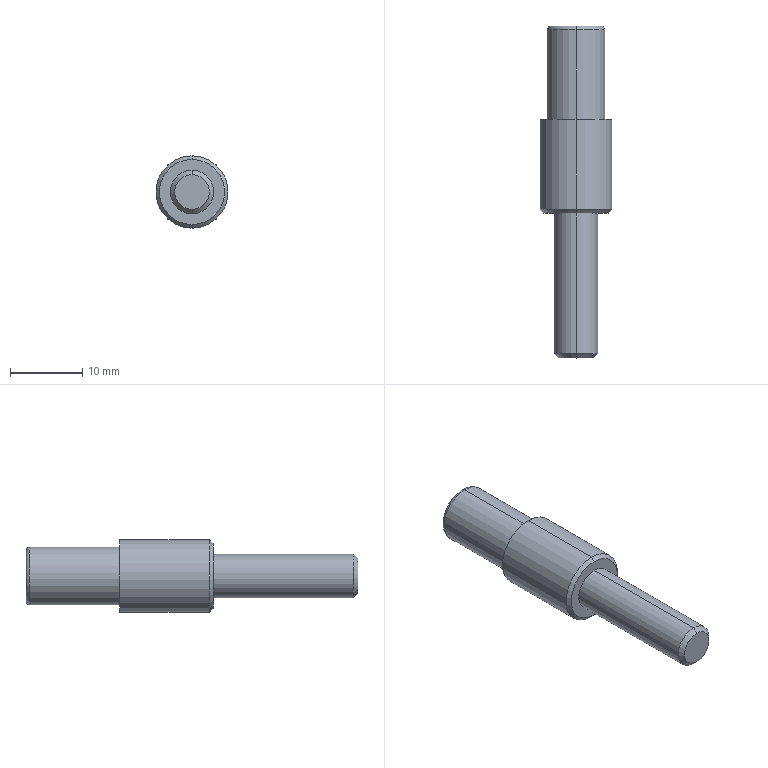Part | STEP file | 11-CLDMC6_20_B_111 | 1 solid | 30 faces | box 10 x 45.8 x 10 mm | volume 2201 mm3 | plane 16 | cone 6 | cylinder 6 | torus 2 | commonest cylinder face diameters 6 x2 8 x2 10 x2
STEP:
#1=CARTESIAN_POINT('',(0.,22.934,0.));
#2=VERTEX_POINT('',#1);
#3=CARTESIAN_POINT('',(0.,23.8,1.5));
#4=VERTEX_POINT('',#3);
#5=CARTESIAN_POINT('',(0.,22.934,0.));
#6=DIRECTION('',(0.,0.5,0.866));
#7=VECTOR('',#6,1000.);
#8=LINE('',#5,#7);
#9=EDGE_CURVE('',#2,#4,#8,.T.);
#10=ORIENTED_EDGE('',*,*,#9,.F.);
#11=CARTESIAN_POINT('',(0.,23.8,-1.5));
#12=VERTEX_POINT('',#11);
#13=CARTESIAN_POINT('',(0.,22.934,0.));
#14=DIRECTION('',(0.,0.5,-0.866));
#15=VECTOR('',#14,1000.);
#16=LINE('',#13,#15);
#17=EDGE_CURVE('',#2,#12,#16,.T.);
#18=ORIENTED_EDGE('',*,*,#17,.T.);
#19=CARTESIAN_POINT('',(-0.75,23.8,-1.299));
#20=VERTEX_POINT('',#19);
#21=CARTESIAN_POINT('',(0.,23.8,0.));
#22=DIRECTION('',(0.,-1.,0.));
#23=DIRECTION('',(0.,0.,1.));
#24=AXIS2_PLACEMENT_3D('',#21,#22,#23);
#25=CIRCLE('',#24,1.5);
#26=EDGE_CURVE('',#20,#12,#25,.T.);
#27=ORIENTED_EDGE('',*,*,#26,.F.);
#28=CARTESIAN_POINT('',(-1.5,23.8,0.));
#29=VERTEX_POINT('',#28);
#30=CARTESIAN_POINT('',(0.,23.8,0.));
#31=DIRECTION('',(0.,-1.,0.));
#32=DIRECTION('',(0.,0.,1.));
#33=AXIS2_PLACEMENT_3D('',#30,#31,#32);
#34=CIRCLE('',#33,1.5);
#35=EDGE_CURVE('',#29,#20,#34,.T.);
#36=ORIENTED_EDGE('',*,*,#35,.F.);
#37=CARTESIAN_POINT('',(-0.75,23.8,1.299));
#38=VERTEX_POINT('',#37);
#39=CARTESIAN_POINT('',(0.,23.8,0.));
#40=DIRECTION('',(0.,-1.,0.));
#41=DIRECTION('',(0.,0.,1.));
#42=AXIS2_PLACEMENT_3D('',#39,#40,#41);
#43=CIRCLE('',#42,1.5);
#44=EDGE_CURVE('',#38,#29,#43,.T.);
#45=ORIENTED_EDGE('',*,*,#44,.F.);
#46=CARTESIAN_POINT('',(0.,23.8,0.));
#47=DIRECTION('',(0.,-1.,0.));
#48=DIRECTION('',(0.,0.,1.));
#49=AXIS2_PLACEMENT_3D('',#46,#47,#48);
#50=CIRCLE('',#49,1.5);
#51=EDGE_CURVE('',#4,#38,#50,.T.);
#52=ORIENTED_EDGE('',*,*,#51,.F.);
#53=EDGE_LOOP('',(#10,#18,#27,#36,#45,#52));
#54=FACE_OUTER_BOUND('',#53,.T.);
#55=CARTESIAN_POINT('',(0.,1022.934,0.));
#56=DIRECTION('',(0.,1.,0.));
#57=DIRECTION('',(0.,0.,1.));
#58=AXIS2_PLACEMENT_3D('',#55,#56,#57);
#59=CONICAL_SURFACE('',#58,1732.051,1.047);
#60=ADVANCED_FACE('',(#54),#59,.F.);
#61=CARTESIAN_POINT('',(0.,-20.,2.387));
#62=VERTEX_POINT('',#61);
#63=CARTESIAN_POINT('',(0.,-20.,-2.387));
#64=VERTEX_POINT('',#63);
#65=CARTESIAN_POINT('',(0.,-20.,0.));
#66=DIRECTION('',(0.,1.,0.));
#67=DIRECTION('',(0.,0.,1.));
#68=AXIS2_PLACEMENT_3D('',#65,#66,#67);
#69=CIRCLE('',#68,2.387);
#70=EDGE_CURVE('',#62,#64,#69,.T.);
#71=ORIENTED_EDGE('',*,*,#70,.T.);
#72=CARTESIAN_POINT('',(0.,-19.387,-3.));
#73=VERTEX_POINT('',#72);
#74=CARTESIAN_POINT('',(0.,-20.,-2.387));
#75=DIRECTION('',(0.,0.7071,-0.7071));
#76=VECTOR('',#75,1000.);
#77=LINE('',#74,#76);
#78=EDGE_CURVE('',#64,#73,#77,.T.);
#79=ORIENTED_EDGE('',*,*,#78,.T.);
#80=CARTESIAN_POINT('',(0.,-19.387,3.));
#81=VERTEX_POINT('',#80);
#82=CARTESIAN_POINT('',(0.,-19.387,0.));
#83=DIRECTION('',(0.,1.,0.));
#84=DIRECTION('',(0.,0.,1.));
#85=AXIS2_PLACEMENT_3D('',#82,#83,#84);
#86=CIRCLE('',#85,3.);
#87=EDGE_CURVE('',#81,#73,#86,.T.);
#88=ORIENTED_EDGE('',*,*,#87,.F.);
#89=CARTESIAN_POINT('',(0.,-20.,2.387));
#90=DIRECTION('',(0.,0.7071,0.7071));
#91=VECTOR('',#90,1000.);
#92=LINE('',#89,#91);
#93=EDGE_CURVE('',#62,#81,#92,.T.);
#94=ORIENTED_EDGE('',*,*,#93,.F.);
#95=EDGE_LOOP('',(#71,#79,#88,#94));
#96=FACE_OUTER_BOUND('',#95,.T.);
#97=CARTESIAN_POINT('',(0.,-20.,0.));
#98=DIRECTION('',(0.,1.,0.));
#99=DIRECTION('',(0.,0.,1.));
#100=AXIS2_PLACEMENT_3D('',#97,#98,#99);
#101=CONICAL_SURFACE('',#100,2.387,0.7854);
#102=ADVANCED_FACE('',(#96),#101,.T.);
#103=ORIENTED_EDGE('',*,*,#87,.T.);
#104=CARTESIAN_POINT('',(0.,0.,-3.));
#105=VERTEX_POINT('',#104);
#106=CARTESIAN_POINT('',(0.,-20.,-3.));
#107=DIRECTION('',(0.,1.,0.));
#108=VECTOR('',#107,1000.);
#109=LINE('',#106,#108);
#110=EDGE_CURVE('',#73,#105,#109,.T.);
#111=ORIENTED_EDGE('',*,*,#110,.T.);
#112=CARTESIAN_POINT('',(0.,0.,3.));
#113=VERTEX_POINT('',#112);
#114=CARTESIAN_POINT('',(0.,0.,0.));
#115=DIRECTION('',(0.,1.,0.));
#116=DIRECTION('',(0.,0.,1.));
#117=AXIS2_PLACEMENT_3D('',#114,#115,#116);
#118=CIRCLE('',#117,3.);
#119=EDGE_CURVE('',#113,#105,#118,.T.);
#120=ORIENTED_EDGE('',*,*,#119,.F.);
#121=CARTESIAN_POINT('',(0.,-20.,3.));
#122=DIRECTION('',(0.,1.,0.));
#123=VECTOR('',#122,1000.);
#124=LINE('',#121,#123);
#125=EDGE_CURVE('',#81,#113,#124,.T.);
#126=ORIENTED_EDGE('',*,*,#125,.F.);
#127=EDGE_LOOP('',(#103,#111,#120,#126));
#128=FACE_OUTER_BOUND('',#127,.T.);
#129=CARTESIAN_POINT('',(0.,-20.,0.));
#130=DIRECTION('',(0.,1.,0.));
#131=DIRECTION('',(0.,0.,1.));
#132=AXIS2_PLACEMENT_3D('',#129,#130,#131);
#133=CYLINDRICAL_SURFACE('',#132,3.);
#134=ADVANCED_FACE('',(#128),#133,.T.);
#135=CARTESIAN_POINT('',(0.,0.,4.5));
#136=VERTEX_POINT('',#135);
#137=CARTESIAN_POINT('',(0.,0.,-4.5));
#138=VERTEX_POINT('',#137);
#139=CARTESIAN_POINT('',(0.,0.,0.));
#140=DIRECTION('',(0.,1.,0.));
#141=DIRECTION('',(0.,0.,1.));
#142=AXIS2_PLACEMENT_3D('',#139,#140,#141);
#143=CIRCLE('',#142,4.5);
#144=EDGE_CURVE('',#136,#138,#143,.T.);
#145=ORIENTED_EDGE('',*,*,#144,.T.);
#146=CARTESIAN_POINT('',(0.,0.5,-5.));
#147=VERTEX_POINT('',#146);
#148=CARTESIAN_POINT('',(0.,0.,-4.5));
#149=DIRECTION('',(0.,0.7071,-0.7071));
#150=VECTOR('',#149,1000.);
#151=LINE('',#148,#150);
#152=EDGE_CURVE('',#138,#147,#151,.T.);
#153=ORIENTED_EDGE('',*,*,#152,.T.);
#154=CARTESIAN_POINT('',(0.,0.5,5.));
#155=VERTEX_POINT('',#154);
#156=CARTESIAN_POINT('',(0.,0.5,0.));
#157=DIRECTION('',(0.,1.,0.));
#158=DIRECTION('',(0.,0.,1.));
#159=AXIS2_PLACEMENT_3D('',#156,#157,#158);
#160=CIRCLE('',#159,5.);
#161=EDGE_CURVE('',#155,#147,#160,.T.);
#162=ORIENTED_EDGE('',*,*,#161,.F.);
#163=CARTESIAN_POINT('',(0.,0.,4.5));
#164=DIRECTION('',(0.,0.7071,0.7071));
#165=VECTOR('',#164,1000.);
#166=LINE('',#163,#165);
#167=EDGE_CURVE('',#136,#155,#166,.T.);
#168=ORIENTED_EDGE('',*,*,#167,.F.);
#169=EDGE_LOOP('',(#145,#153,#162,#168));
#170=FACE_OUTER_BOUND('',#169,.T.);
#171=CARTESIAN_POINT('',(0.,0.,0.));
#172=DIRECTION('',(0.,1.,0.));
#173=DIRECTION('',(0.,0.,1.));
#174=AXIS2_PLACEMENT_3D('',#171,#172,#173);
#175=CONICAL_SURFACE('',#174,4.5,0.7854);
#176=ADVANCED_FACE('',(#170),#175,.T.);
#177=ORIENTED_EDGE('',*,*,#161,.T.);
#178=CARTESIAN_POINT('',(0.,12.9,-5.));
#179=VERTEX_POINT('',#178);
#180=CARTESIAN_POINT('',(0.,-20.,-5.));
#181=DIRECTION('',(0.,1.,0.));
#182=VECTOR('',#181,1000.);
#183=LINE('',#180,#182);
#184=EDGE_CURVE('',#147,#179,#183,.T.);
#185=ORIENTED_EDGE('',*,*,#184,.T.);
#186=CARTESIAN_POINT('',(0.,12.9,5.));
#187=VERTEX_POINT('',#186);
#188=CARTESIAN_POINT('',(0.,12.9,0.));
#189=DIRECTION('',(0.,1.,0.));
#190=DIRECTION('',(0.,0.,1.));
#191=AXIS2_PLACEMENT_3D('',#188,#189,#190);
#192=CIRCLE('',#191,5.);
#193=EDGE_CURVE('',#187,#179,#192,.T.);
#194=ORIENTED_EDGE('',*,*,#193,.F.);
#195=CARTESIAN_POINT('',(0.,-20.,5.));
#196=DIRECTION('',(0.,1.,0.));
#197=VECTOR('',#196,1000.);
#198=LINE('',#195,#197);
#199=EDGE_CURVE('',#155,#187,#198,.T.);
#200=ORIENTED_EDGE('',*,*,#199,.F.);
#201=EDGE_LOOP('',(#177,#185,#194,#200));
#202=FACE_OUTER_BOUND('',#201,.T.);
#203=CARTESIAN_POINT('',(0.,-20.,0.));
#204=DIRECTION('',(0.,1.,0.));
#205=DIRECTION('',(0.,0.,1.));
#206=AXIS2_PLACEMENT_3D('',#203,#204,#205);
#207=CYLINDRICAL_SURFACE('',#206,5.);
#208=ADVANCED_FACE('',(#202),#207,.T.);
#209=CARTESIAN_POINT('',(0.,12.9,4.));
#210=VERTEX_POINT('',#209);
#211=CARTESIAN_POINT('',(0.,12.9,-4.));
#212=VERTEX_POINT('',#211);
#213=CARTESIAN_POINT('',(0.,12.9,0.));
#214=DIRECTION('',(0.,1.,0.));
#215=DIRECTION('',(0.,0.,1.));
#216=AXIS2_PLACEMENT_3D('',#213,#214,#215);
#217=CIRCLE('',#216,4.);
#218=EDGE_CURVE('',#210,#212,#217,.T.);
#219=ORIENTED_EDGE('',*,*,#218,.T.);
#220=CARTESIAN_POINT('',(0.,25.3,-4.));
#221=VERTEX_POINT('',#220);
#222=CARTESIAN_POINT('',(0.,-20.,-4.));
#223=DIRECTION('',(0.,1.,0.));
#224=VECTOR('',#223,1000.);
#225=LINE('',#222,#224);
#226=EDGE_CURVE('',#212,#221,#225,.T.);
#227=ORIENTED_EDGE('',*,*,#226,.T.);
#228=CARTESIAN_POINT('',(0.,25.3,4.));
#229=VERTEX_POINT('',#228);
#230=CARTESIAN_POINT('',(0.,25.3,0.));
#231=DIRECTION('',(0.,1.,0.));
#232=DIRECTION('',(0.,0.,1.));
#233=AXIS2_PLACEMENT_3D('',#230,#231,#232);
#234=CIRCLE('',#233,4.);
#235=EDGE_CURVE('',#229,#221,#234,.T.);
#236=ORIENTED_EDGE('',*,*,#235,.F.);
#237=CARTESIAN_POINT('',(0.,-20.,4.));
#238=DIRECTION('',(0.,1.,0.));
#239=VECTOR('',#238,1000.);
#240=LINE('',#237,#239);
#241=EDGE_CURVE('',#210,#229,#240,.T.);
#242=ORIENTED_EDGE('',*,*,#241,.F.);
#243=EDGE_LOOP('',(#219,#227,#236,#242));
#244=FACE_OUTER_BOUND('',#243,.T.);
#245=CARTESIAN_POINT('',(0.,-20.,0.));
#246=DIRECTION('',(0.,1.,0.));
#247=DIRECTION('',(0.,0.,1.));
#248=AXIS2_PLACEMENT_3D('',#245,#246,#247);
#249=CYLINDRICAL_SURFACE('',#248,4.);
#250=ADVANCED_FACE('',(#244),#249,.T.);
#251=ORIENTED_EDGE('',*,*,#235,.T.);
#252=CARTESIAN_POINT('',(0.,25.8,-3.5));
#253=VERTEX_POINT('',#252);
#254=CARTESIAN_POINT('',(0.,25.3,-3.5));
#255=DIRECTION('',(1.,0.,0.));
#256=DIRECTION('',(0.,0.,-1.));
#257=AXIS2_PLACEMENT_3D('',#254,#255,#256);
#258=CIRCLE('',#257,0.5);
#259=EDGE_CURVE('',#221,#253,#258,.T.);
#260=ORIENTED_EDGE('',*,*,#259,.T.);
#261=CARTESIAN_POINT('',(0.,25.8,3.5));
#262=VERTEX_POINT('',#261);
#263=CARTESIAN_POINT('',(0.,25.8,0.));
#264=DIRECTION('',(0.,1.,0.));
#265=DIRECTION('',(0.,0.,1.));
#266=AXIS2_PLACEMENT_3D('',#263,#264,#265);
#267=CIRCLE('',#266,3.5);
#268=EDGE_CURVE('',#262,#253,#267,.T.);
#269=ORIENTED_EDGE('',*,*,#268,.F.);
#270=CARTESIAN_POINT('',(0.,25.3,3.5));
#271=DIRECTION('',(-1.,0.,0.));
#272=DIRECTION('',(0.,0.,1.));
#273=AXIS2_PLACEMENT_3D('',#270,#271,#272);
#274=CIRCLE('',#273,0.5);
#275=EDGE_CURVE('',#229,#262,#274,.T.);
#276=ORIENTED_EDGE('',*,*,#275,.F.);
#277=EDGE_LOOP('',(#251,#260,#269,#276));
#278=FACE_OUTER_BOUND('',#277,.T.);
#279=CARTESIAN_POINT('',(0.,25.3,0.));
#280=DIRECTION('',(0.,1.,0.));
#281=DIRECTION('',(0.,0.,1.));
#282=AXIS2_PLACEMENT_3D('',#279,#280,#281);
#283=TOROIDAL_SURFACE('',#282,3.5,0.5);
#284=ADVANCED_FACE('',(#278),#283,.T.);
#285=CARTESIAN_POINT('',(-1.5,23.8,0.866));
#286=VERTEX_POINT('',#285);
#287=CARTESIAN_POINT('',(-1.5,23.8,0.866));
#288=DIRECTION('',(0.866,0.,0.5));
#289=VECTOR('',#288,1000.);
#290=LINE('',#287,#289);
#291=EDGE_CURVE('',#286,#38,#290,.T.);
#292=ORIENTED_EDGE('',*,*,#291,.T.);
#293=ORIENTED_EDGE('',*,*,#44,.T.);
#294=CARTESIAN_POINT('',(-1.5,23.8,-0.866));
#295=DIRECTION('',(0.,0.,1.));
#296=VECTOR('',#295,1000.);
#297=LINE('',#294,#296);
#298=EDGE_CURVE('',#29,#286,#297,.T.);
#299=ORIENTED_EDGE('',*,*,#298,.T.);
#300=EDGE_LOOP('',(#292,#293,#299));
#301=FACE_OUTER_BOUND('',#300,.T.);
#302=CARTESIAN_POINT('',(-1.5,23.8,-0.866));
#303=DIRECTION('',(0.,1.,0.));
#304=DIRECTION('',(0.,0.,1.));
#305=AXIS2_PLACEMENT_3D('',#302,#303,#304);
#306=PLANE('',#305);
#307=ADVANCED_FACE('',(#301),#306,.T.);
#308=CARTESIAN_POINT('',(-1.5,23.8,-0.866));
#309=VERTEX_POINT('',#308);
#310=CARTESIAN_POINT('',(-1.5,23.8,-0.866));
#311=DIRECTION('',(0.,0.,1.));
#312=VECTOR('',#311,1000.);
#313=LINE('',#310,#312);
#314=EDGE_CURVE('',#309,#29,#313,.T.);
#315=ORIENTED_EDGE('',*,*,#314,.T.);
#316=ORIENTED_EDGE('',*,*,#35,.T.);
#317=CARTESIAN_POINT('',(0.,23.8,-1.732));
#318=DIRECTION('',(-0.866,0.,0.5));
#319=VECTOR('',#318,1000.);
#320=LINE('',#317,#319);
#321=EDGE_CURVE('',#20,#309,#320,.T.);
#322=ORIENTED_EDGE('',*,*,#321,.T.);
#323=EDGE_LOOP('',(#315,#316,#322));
#324=FACE_OUTER_BOUND('',#323,.T.);
#325=CARTESIAN_POINT('',(-1.5,23.8,-0.866));
#326=DIRECTION('',(0.,1.,0.));
#327=DIRECTION('',(0.,0.,1.));
#328=AXIS2_PLACEMENT_3D('',#325,#326,#327);
#329=PLANE('',#328);
#330=ADVANCED_FACE('',(#324),#329,.T.);
#331=CARTESIAN_POINT('',(0.,23.8,-1.732));
#332=VERTEX_POINT('',#331);
#333=CARTESIAN_POINT('',(0.,23.8,-1.732));
#334=DIRECTION('',(-0.866,0.,0.5));
#335=VECTOR('',#334,1000.);
#336=LINE('',#333,#335);
#337=EDGE_CURVE('',#332,#20,#336,.T.);
#338=ORIENTED_EDGE('',*,*,#337,.T.);
#339=ORIENTED_EDGE('',*,*,#26,.T.);
#340=CARTESIAN_POINT('',(0.75,23.8,-1.299));
#341=VERTEX_POINT('',#340);
#342=CARTESIAN_POINT('',(0.,23.8,0.));
#343=DIRECTION('',(0.,-1.,0.));
#344=DIRECTION('',(0.,0.,1.));
#345=AXIS2_PLACEMENT_3D('',#342,#343,#344);
#346=CIRCLE('',#345,1.5);
#347=EDGE_CURVE('',#12,#341,#346,.T.);
#348=ORIENTED_EDGE('',*,*,#347,.T.);
#349=CARTESIAN_POINT('',(1.5,23.8,-0.866));
#350=DIRECTION('',(-0.866,0.,-0.5));
#351=VECTOR('',#350,1000.);
#352=LINE('',#349,#351);
#353=EDGE_CURVE('',#341,#332,#352,.T.);
#354=ORIENTED_EDGE('',*,*,#353,.T.);
#355=EDGE_LOOP('',(#338,#339,#348,#354));
#356=FACE_OUTER_BOUND('',#355,.T.);
#357=CARTESIAN_POINT('',(-1.5,23.8,-0.866));
#358=DIRECTION('',(0.,1.,0.));
#359=DIRECTION('',(0.,0.,1.));
#360=AXIS2_PLACEMENT_3D('',#357,#358,#359);
#361=PLANE('',#360);
#362=ADVANCED_FACE('',(#356),#361,.T.);
#363=CARTESIAN_POINT('',(1.5,23.8,-0.866));
#364=VERTEX_POINT('',#363);
#365=CARTESIAN_POINT('',(1.5,23.8,-0.866));
#366=DIRECTION('',(-0.866,0.,-0.5));
#367=VECTOR('',#366,1000.);
#368=LINE('',#365,#367);
#369=EDGE_CURVE('',#364,#341,#368,.T.);
#370=ORIENTED_EDGE('',*,*,#369,.T.);
#371=CARTESIAN_POINT('',(1.5,23.8,0.));
#372=VERTEX_POINT('',#371);
#373=CARTESIAN_POINT('',(0.,23.8,0.));
#374=DIRECTION('',(0.,-1.,0.));
#375=DIRECTION('',(0.,0.,1.));
#376=AXIS2_PLACEMENT_3D('',#373,#374,#375);
#377=CIRCLE('',#376,1.5);
#378=EDGE_CURVE('',#341,#372,#377,.T.);
#379=ORIENTED_EDGE('',*,*,#378,.T.);
#380=CARTESIAN_POINT('',(1.5,23.8,0.866));
#381=DIRECTION('',(0.,0.,-1.));
#382=VECTOR('',#381,1000.);
#383=LINE('',#380,#382);
#384=EDGE_CURVE('',#372,#364,#383,.T.);
#385=ORIENTED_EDGE('',*,*,#384,.T.);
#386=EDGE_LOOP('',(#370,#379,#385));
#387=FACE_OUTER_BOUND('',#386,.T.);
#388=CARTESIAN_POINT('',(-1.5,23.8,-0.866));
#389=DIRECTION('',(0.,1.,0.));
#390=DIRECTION('',(0.,0.,1.));
#391=AXIS2_PLACEMENT_3D('',#388,#389,#390);
#392=PLANE('',#391);
#393=ADVANCED_FACE('',(#387),#392,.T.);
#394=CARTESIAN_POINT('',(1.5,23.8,0.866));
#395=VERTEX_POINT('',#394);
#396=CARTESIAN_POINT('',(1.5,23.8,0.866));
#397=DIRECTION('',(0.,0.,-1.));
#398=VECTOR('',#397,1000.);
#399=LINE('',#396,#398);
#400=EDGE_CURVE('',#395,#372,#399,.T.);
#401=ORIENTED_EDGE('',*,*,#400,.T.);
#402=CARTESIAN_POINT('',(0.75,23.8,1.299));
#403=VERTEX_POINT('',#402);
#404=CARTESIAN_POINT('',(0.,23.8,0.));
#405=DIRECTION('',(0.,1.,0.));
#406=DIRECTION('',(0.,0.,1.));
#407=AXIS2_PLACEMENT_3D('',#404,#405,#406);
#408=CIRCLE('',#407,1.5);
#409=EDGE_CURVE('',#403,#372,#408,.T.);
#410=ORIENTED_EDGE('',*,*,#409,.F.);
#411=CARTESIAN_POINT('',(0.,23.8,1.732));
#412=DIRECTION('',(0.866,0.,-0.5));
#413=VECTOR('',#412,1000.);
#414=LINE('',#411,#413);
#415=EDGE_CURVE('',#403,#395,#414,.T.);
#416=ORIENTED_EDGE('',*,*,#415,.T.);
#417=EDGE_LOOP('',(#401,#410,#416));
#418=FACE_OUTER_BOUND('',#417,.T.);
#419=CARTESIAN_POINT('',(-1.5,23.8,-0.866));
#420=DIRECTION('',(0.,1.,0.));
#421=DIRECTION('',(0.,0.,1.));
#422=AXIS2_PLACEMENT_3D('',#419,#420,#421);
#423=PLANE('',#422);
#424=ADVANCED_FACE('',(#418),#423,.T.);
#425=CARTESIAN_POINT('',(0.,23.8,1.732));
#426=VERTEX_POINT('',#425);
#427=CARTESIAN_POINT('',(0.,23.8,1.732));
#428=DIRECTION('',(0.866,0.,-0.5));
#429=VECTOR('',#428,1000.);
#430=LINE('',#427,#429);
#431=EDGE_CURVE('',#426,#403,#430,.T.);
#432=ORIENTED_EDGE('',*,*,#431,.T.);
#433=CARTESIAN_POINT('',(0.,23.8,0.));
#434=DIRECTION('',(0.,-1.,0.));
#435=DIRECTION('',(0.,0.,1.));
#436=AXIS2_PLACEMENT_3D('',#433,#434,#435);
#437=CIRCLE('',#436,1.5);
#438=EDGE_CURVE('',#403,#4,#437,.T.);
#439=ORIENTED_EDGE('',*,*,#438,.T.);
#440=ORIENTED_EDGE('',*,*,#51,.T.);
#441=CARTESIAN_POINT('',(-1.5,23.8,0.866));
#442=DIRECTION('',(0.866,0.,0.5));
#443=VECTOR('',#442,1000.);
#444=LINE('',#441,#443);
#445=EDGE_CURVE('',#38,#426,#444,.T.);
#446=ORIENTED_EDGE('',*,*,#445,.T.);
#447=EDGE_LOOP('',(#432,#439,#440,#446));
#448=FACE_OUTER_BOUND('',#447,.T.);
#449=CARTESIAN_POINT('',(-1.5,23.8,-0.866));
#450=DIRECTION('',(0.,1.,0.));
#451=DIRECTION('',(0.,0.,1.));
#452=AXIS2_PLACEMENT_3D('',#449,#450,#451);
#453=PLANE('',#452);
#454=ADVANCED_FACE('',(#448),#453,.T.);
#455=ORIENTED_EDGE('',*,*,#268,.T.);
#456=CARTESIAN_POINT('',(0.,25.8,0.));
#457=DIRECTION('',(0.,1.,0.));
#458=DIRECTION('',(0.,0.,1.));
#459=AXIS2_PLACEMENT_3D('',#456,#457,#458);
#460=CIRCLE('',#459,3.5);
#461=EDGE_CURVE('',#253,#262,#460,.T.);
#462=ORIENTED_EDGE('',*,*,#461,.T.);
#463=EDGE_LOOP('',(#455,#462));
#464=FACE_OUTER_BOUND('',#463,.T.);
#465=CARTESIAN_POINT('',(0.,25.8,-1.732));
#466=VERTEX_POINT('',#465);
#467=CARTESIAN_POINT('',(-1.5,25.8,-0.866));
#468=VERTEX_POINT('',#467);
#469=CARTESIAN_POINT('',(-0.75,25.8,-1.299));
#470=DIRECTION('',(-0.866,0.,0.5));
#471=VECTOR('',#470,1000.);
#472=LINE('',#469,#471);
#473=EDGE_CURVE('',#466,#468,#472,.T.);
#474=ORIENTED_EDGE('',*,*,#473,.F.);
#475=CARTESIAN_POINT('',(1.5,25.8,-0.866));
#476=VERTEX_POINT('',#475);
#477=CARTESIAN_POINT('',(0.75,25.8,-1.299));
#478=DIRECTION('',(-0.866,0.,-0.5));
#479=VECTOR('',#478,1000.);
#480=LINE('',#477,#479);
#481=EDGE_CURVE('',#476,#466,#480,.T.);
#482=ORIENTED_EDGE('',*,*,#481,.F.);
#483=CARTESIAN_POINT('',(1.5,25.8,0.866));
#484=VERTEX_POINT('',#483);
#485=CARTESIAN_POINT('',(1.5,25.8,0.));
#486=DIRECTION('',(0.,0.,-1.));
#487=VECTOR('',#486,1000.);
#488=LINE('',#485,#487);
#489=EDGE_CURVE('',#484,#476,#488,.T.);
#490=ORIENTED_EDGE('',*,*,#489,.F.);
#491=CARTESIAN_POINT('',(0.,25.8,1.732));
#492=VERTEX_POINT('',#491);
#493=CARTESIAN_POINT('',(0.75,25.8,1.299));
#494=DIRECTION('',(0.866,0.,-0.5));
#495=VECTOR('',#494,1000.);
#496=LINE('',#493,#495);
#497=EDGE_CURVE('',#492,#484,#496,.T.);
#498=ORIENTED_EDGE('',*,*,#497,.F.);
#499=CARTESIAN_POINT('',(-1.5,25.8,0.866));
#500=VERTEX_POINT('',#499);
#501=CARTESIAN_POINT('',(-0.75,25.8,1.299));
#502=DIRECTION('',(0.866,0.,0.5));
#503=VECTOR('',#502,1000.);
#504=LINE('',#501,#503);
#505=EDGE_CURVE('',#500,#492,#504,.T.);
#506=ORIENTED_EDGE('',*,*,#505,.F.);
#507=CARTESIAN_POINT('',(-1.5,25.8,0.));
#508=DIRECTION('',(0.,0.,1.));
#509=VECTOR('',#508,1000.);
#510=LINE('',#507,#509);
#511=EDGE_CURVE('',#468,#500,#510,.T.);
#512=ORIENTED_EDGE('',*,*,#511,.F.);
#513=EDGE_LOOP('',(#474,#482,#490,#498,#506,#512));
#514=FACE_BOUND('',#513,.T.);
#515=CARTESIAN_POINT('',(0.,25.8,0.));
#516=DIRECTION('',(0.,-1.,0.));
#517=DIRECTION('',(0.,0.,-1.));
#518=AXIS2_PLACEMENT_3D('',#515,#516,#517);
#519=PLANE('',#518);
#520=ADVANCED_FACE('',(#464,#514),#519,.F.);
#521=ORIENTED_EDGE('',*,*,#259,.F.);
#522=CARTESIAN_POINT('',(0.,25.3,0.));
#523=DIRECTION('',(0.,1.,0.));
#524=DIRECTION('',(0.,0.,1.));
#525=AXIS2_PLACEMENT_3D('',#522,#523,#524);
#526=CIRCLE('',#525,4.);
#527=EDGE_CURVE('',#221,#229,#526,.T.);
#528=ORIENTED_EDGE('',*,*,#527,.T.);
#529=ORIENTED_EDGE('',*,*,#275,.T.);
#530=ORIENTED_EDGE('',*,*,#461,.F.);
#531=EDGE_LOOP('',(#521,#528,#529,#530));
#532=FACE_OUTER_BOUND('',#531,.T.);
#533=CARTESIAN_POINT('',(0.,25.3,0.));
#534=DIRECTION('',(0.,1.,0.));
#535=DIRECTION('',(0.,0.,1.));
#536=AXIS2_PLACEMENT_3D('',#533,#534,#535);
#537=TOROIDAL_SURFACE('',#536,3.5,0.5);
#538=ADVANCED_FACE('',(#532),#537,.T.);
#539=ORIENTED_EDGE('',*,*,#226,.F.);
#540=CARTESIAN_POINT('',(0.,12.9,0.));
#541=DIRECTION('',(0.,1.,0.));
#542=DIRECTION('',(0.,0.,1.));
#543=AXIS2_PLACEMENT_3D('',#540,#541,#542);
#544=CIRCLE('',#543,4.);
#545=EDGE_CURVE('',#212,#210,#544,.T.);
#546=ORIENTED_EDGE('',*,*,#545,.T.);
#547=ORIENTED_EDGE('',*,*,#241,.T.);
#548=ORIENTED_EDGE('',*,*,#527,.F.);
#549=EDGE_LOOP('',(#539,#546,#547,#548));
#550=FACE_OUTER_BOUND('',#549,.T.);
#551=CARTESIAN_POINT('',(0.,-20.,0.));
#552=DIRECTION('',(0.,1.,0.));
#553=DIRECTION('',(0.,0.,1.));
#554=AXIS2_PLACEMENT_3D('',#551,#552,#553);
#555=CYLINDRICAL_SURFACE('',#554,4.);
#556=ADVANCED_FACE('',(#550),#555,.T.);
#557=ORIENTED_EDGE('',*,*,#218,.F.);
#558=ORIENTED_EDGE('',*,*,#545,.F.);
#559=EDGE_LOOP('',(#557,#558));
#560=FACE_BOUND('',#559,.T.);
#561=ORIENTED_EDGE('',*,*,#193,.T.);
#562=CARTESIAN_POINT('',(0.,12.9,0.));
#563=DIRECTION('',(0.,1.,0.));
#564=DIRECTION('',(0.,0.,1.));
#565=AXIS2_PLACEMENT_3D('',#562,#563,#564);
#566=CIRCLE('',#565,5.);
#567=EDGE_CURVE('',#179,#187,#566,.T.);
#568=ORIENTED_EDGE('',*,*,#567,.T.);
#569=EDGE_LOOP('',(#561,#568));
#570=FACE_OUTER_BOUND('',#569,.T.);
#571=CARTESIAN_POINT('',(4.,12.9,0.));
#572=DIRECTION('',(0.,-1.,0.));
#573=DIRECTION('',(0.,0.,-1.));
#574=AXIS2_PLACEMENT_3D('',#571,#572,#573);
#575=PLANE('',#574);
#576=ADVANCED_FACE('',(#560,#570),#575,.F.);
#577=ORIENTED_EDGE('',*,*,#184,.F.);
#578=CARTESIAN_POINT('',(0.,0.5,0.));
#579=DIRECTION('',(0.,1.,0.));
#580=DIRECTION('',(0.,0.,1.));
#581=AXIS2_PLACEMENT_3D('',#578,#579,#580);
#582=CIRCLE('',#581,5.);
#583=EDGE_CURVE('',#147,#155,#582,.T.);
#584=ORIENTED_EDGE('',*,*,#583,.T.);
#585=ORIENTED_EDGE('',*,*,#199,.T.);
#586=ORIENTED_EDGE('',*,*,#567,.F.);
#587=EDGE_LOOP('',(#577,#584,#585,#586));
#588=FACE_OUTER_BOUND('',#587,.T.);
#589=CARTESIAN_POINT('',(0.,-20.,0.));
#590=DIRECTION('',(0.,1.,0.));
#591=DIRECTION('',(0.,0.,1.));
#592=AXIS2_PLACEMENT_3D('',#589,#590,#591);
#593=CYLINDRICAL_SURFACE('',#592,5.);
#594=ADVANCED_FACE('',(#588),#593,.T.);
#595=ORIENTED_EDGE('',*,*,#152,.F.);
#596=CARTESIAN_POINT('',(0.,0.,0.));
#597=DIRECTION('',(0.,1.,0.));
#598=DIRECTION('',(0.,0.,1.));
#599=AXIS2_PLACEMENT_3D('',#596,#597,#598);
#600=CIRCLE('',#599,4.5);
#601=EDGE_CURVE('',#138,#136,#600,.T.);
#602=ORIENTED_EDGE('',*,*,#601,.T.);
#603=ORIENTED_EDGE('',*,*,#167,.T.);
#604=ORIENTED_EDGE('',*,*,#583,.F.);
#605=EDGE_LOOP('',(#595,#602,#603,#604));
#606=FACE_OUTER_BOUND('',#605,.T.);
#607=CARTESIAN_POINT('',(0.,0.,0.));
#608=DIRECTION('',(0.,1.,0.));
#609=DIRECTION('',(0.,0.,1.));
#610=AXIS2_PLACEMENT_3D('',#607,#608,#609);
#611=CONICAL_SURFACE('',#610,4.5,0.7854);
#612=ADVANCED_FACE('',(#606),#611,.T.);
#613=ORIENTED_EDGE('',*,*,#144,.F.);
#614=ORIENTED_EDGE('',*,*,#601,.F.);
#615=EDGE_LOOP('',(#613,#614));
#616=FACE_OUTER_BOUND('',#615,.T.);
#617=ORIENTED_EDGE('',*,*,#119,.T.);
#618=CARTESIAN_POINT('',(0.,0.,0.));
#619=DIRECTION('',(0.,1.,0.));
#620=DIRECTION('',(0.,0.,1.));
#621=AXIS2_PLACEMENT_3D('',#618,#619,#620);
#622=CIRCLE('',#621,3.);
#623=EDGE_CURVE('',#105,#113,#622,.T.);
#624=ORIENTED_EDGE('',*,*,#623,.T.);
#625=EDGE_LOOP('',(#617,#624));
#626=FACE_BOUND('',#625,.T.);
#627=CARTESIAN_POINT('',(4.5,0.,0.));
#628=DIRECTION('',(0.,1.,0.));
#629=DIRECTION('',(0.,0.,1.));
#630=AXIS2_PLACEMENT_3D('',#627,#628,#629);
#631=PLANE('',#630);
#632=ADVANCED_FACE('',(#616,#626),#631,.F.);
#633=ORIENTED_EDGE('',*,*,#110,.F.);
#634=CARTESIAN_POINT('',(0.,-19.387,0.));
#635=DIRECTION('',(0.,1.,0.));
#636=DIRECTION('',(0.,0.,1.));
#637=AXIS2_PLACEMENT_3D('',#634,#635,#636);
#638=CIRCLE('',#637,3.);
#639=EDGE_CURVE('',#73,#81,#638,.T.);
#640=ORIENTED_EDGE('',*,*,#639,.T.);
#641=ORIENTED_EDGE('',*,*,#125,.T.);
#642=ORIENTED_EDGE('',*,*,#623,.F.);
#643=EDGE_LOOP('',(#633,#640,#641,#642));
#644=FACE_OUTER_BOUND('',#643,.T.);
#645=CARTESIAN_POINT('',(0.,-20.,0.));
#646=DIRECTION('',(0.,1.,0.));
#647=DIRECTION('',(0.,0.,1.));
#648=AXIS2_PLACEMENT_3D('',#645,#646,#647);
#649=CYLINDRICAL_SURFACE('',#648,3.);
#650=ADVANCED_FACE('',(#644),#649,.T.);
#651=ORIENTED_EDGE('',*,*,#78,.F.);
#652=CARTESIAN_POINT('',(0.,-20.,0.));
#653=DIRECTION('',(0.,1.,0.));
#654=DIRECTION('',(0.,0.,1.));
#655=AXIS2_PLACEMENT_3D('',#652,#653,#654);
#656=CIRCLE('',#655,2.387);
#657=EDGE_CURVE('',#64,#62,#656,.T.);
#658=ORIENTED_EDGE('',*,*,#657,.T.);
#659=ORIENTED_EDGE('',*,*,#93,.T.);
#660=ORIENTED_EDGE('',*,*,#639,.F.);
#661=EDGE_LOOP('',(#651,#658,#659,#660));
#662=FACE_OUTER_BOUND('',#661,.T.);
#663=CARTESIAN_POINT('',(0.,-20.,0.));
#664=DIRECTION('',(0.,1.,0.));
#665=DIRECTION('',(0.,0.,1.));
#666=AXIS2_PLACEMENT_3D('',#663,#664,#665);
#667=CONICAL_SURFACE('',#666,2.387,0.7854);
#668=ADVANCED_FACE('',(#662),#667,.T.);
#669=ORIENTED_EDGE('',*,*,#70,.F.);
#670=ORIENTED_EDGE('',*,*,#657,.F.);
#671=EDGE_LOOP('',(#669,#670));
#672=FACE_OUTER_BOUND('',#671,.T.);
#673=CARTESIAN_POINT('',(2.387,-20.,0.));
#674=DIRECTION('',(0.,1.,0.));
#675=DIRECTION('',(0.,0.,1.));
#676=AXIS2_PLACEMENT_3D('',#673,#674,#675);
#677=PLANE('',#676);
#678=ADVANCED_FACE('',(#672),#677,.F.);
#679=ORIENTED_EDGE('',*,*,#321,.F.);
#680=ORIENTED_EDGE('',*,*,#337,.F.);
#681=CARTESIAN_POINT('',(0.,27.8,-1.732));
#682=DIRECTION('',(0.,-1.,0.));
#683=VECTOR('',#682,1000.);
#684=LINE('',#681,#683);
#685=EDGE_CURVE('',#466,#332,#684,.T.);
#686=ORIENTED_EDGE('',*,*,#685,.F.);
#687=ORIENTED_EDGE('',*,*,#473,.T.);
#688=CARTESIAN_POINT('',(-1.5,27.8,-0.866));
#689=DIRECTION('',(0.,-1.,0.));
#690=VECTOR('',#689,1000.);
#691=LINE('',#688,#690);
#692=EDGE_CURVE('',#468,#309,#691,.T.);
#693=ORIENTED_EDGE('',*,*,#692,.T.);
#694=EDGE_LOOP('',(#679,#680,#686,#687,#693));
#695=FACE_OUTER_BOUND('',#694,.T.);
#696=CARTESIAN_POINT('',(0.,27.8,-1.732));
#697=DIRECTION('',(0.5,0.,0.866));
#698=DIRECTION('',(0.866,0.,-0.5));
#699=AXIS2_PLACEMENT_3D('',#696,#697,#698);
#700=PLANE('',#699);
#701=ADVANCED_FACE('',(#695),#700,.T.);
#702=ORIENTED_EDGE('',*,*,#298,.F.);
#703=ORIENTED_EDGE('',*,*,#314,.F.);
#704=ORIENTED_EDGE('',*,*,#692,.F.);
#705=ORIENTED_EDGE('',*,*,#511,.T.);
#706=CARTESIAN_POINT('',(-1.5,27.8,0.866));
#707=DIRECTION('',(0.,-1.,0.));
#708=VECTOR('',#707,1000.);
#709=LINE('',#706,#708);
#710=EDGE_CURVE('',#500,#286,#709,.T.);
#711=ORIENTED_EDGE('',*,*,#710,.T.);
#712=EDGE_LOOP('',(#702,#703,#704,#705,#711));
#713=FACE_OUTER_BOUND('',#712,.T.);
#714=CARTESIAN_POINT('',(-1.5,27.8,-0.866));
#715=DIRECTION('',(1.,0.,0.));
#716=DIRECTION('',(0.,0.,-1.));
#717=AXIS2_PLACEMENT_3D('',#714,#715,#716);
#718=PLANE('',#717);
#719=ADVANCED_FACE('',(#713),#718,.T.);
#720=ORIENTED_EDGE('',*,*,#445,.F.);
#721=ORIENTED_EDGE('',*,*,#291,.F.);
#722=ORIENTED_EDGE('',*,*,#710,.F.);
#723=ORIENTED_EDGE('',*,*,#505,.T.);
#724=CARTESIAN_POINT('',(0.,27.8,1.732));
#725=DIRECTION('',(0.,-1.,0.));
#726=VECTOR('',#725,1000.);
#727=LINE('',#724,#726);
#728=EDGE_CURVE('',#492,#426,#727,.T.);
#729=ORIENTED_EDGE('',*,*,#728,.T.);
#730=EDGE_LOOP('',(#720,#721,#722,#723,#729));
#731=FACE_OUTER_BOUND('',#730,.T.);
#732=CARTESIAN_POINT('',(-1.5,27.8,0.866));
#733=DIRECTION('',(0.5,0.,-0.866));
#734=DIRECTION('',(-0.866,0.,-0.5));
#735=AXIS2_PLACEMENT_3D('',#732,#733,#734);
#736=PLANE('',#735);
#737=ADVANCED_FACE('',(#731),#736,.T.);
#738=ORIENTED_EDGE('',*,*,#415,.F.);
#739=ORIENTED_EDGE('',*,*,#431,.F.);
#740=ORIENTED_EDGE('',*,*,#728,.F.);
#741=ORIENTED_EDGE('',*,*,#497,.T.);
#742=CARTESIAN_POINT('',(1.5,27.8,0.866));
#743=DIRECTION('',(0.,-1.,0.));
#744=VECTOR('',#743,1000.);
#745=LINE('',#742,#744);
#746=EDGE_CURVE('',#484,#395,#745,.T.);
#747=ORIENTED_EDGE('',*,*,#746,.T.);
#748=EDGE_LOOP('',(#738,#739,#740,#741,#747));
#749=FACE_OUTER_BOUND('',#748,.T.);
#750=CARTESIAN_POINT('',(0.,27.8,1.732));
#751=DIRECTION('',(-0.5,0.,-0.866));
#752=DIRECTION('',(-0.866,0.,0.5));
#753=AXIS2_PLACEMENT_3D('',#750,#751,#752);
#754=PLANE('',#753);
#755=ADVANCED_FACE('',(#749),#754,.T.);
#756=ORIENTED_EDGE('',*,*,#384,.F.);
#757=ORIENTED_EDGE('',*,*,#400,.F.);
#758=ORIENTED_EDGE('',*,*,#746,.F.);
#759=ORIENTED_EDGE('',*,*,#489,.T.);
#760=CARTESIAN_POINT('',(1.5,27.8,-0.866));
#761=DIRECTION('',(0.,-1.,0.));
#762=VECTOR('',#761,1000.);
#763=LINE('',#760,#762);
#764=EDGE_CURVE('',#476,#364,#763,.T.);
#765=ORIENTED_EDGE('',*,*,#764,.T.);
#766=EDGE_LOOP('',(#756,#757,#758,#759,#765));
#767=FACE_OUTER_BOUND('',#766,.T.);
#768=CARTESIAN_POINT('',(1.5,27.8,0.866));
#769=DIRECTION('',(-1.,0.,0.));
#770=DIRECTION('',(0.,0.,1.));
#771=AXIS2_PLACEMENT_3D('',#768,#769,#770);
#772=PLANE('',#771);
#773=ADVANCED_FACE('',(#767),#772,.T.);
#774=ORIENTED_EDGE('',*,*,#353,.F.);
#775=ORIENTED_EDGE('',*,*,#369,.F.);
#776=ORIENTED_EDGE('',*,*,#764,.F.);
#777=ORIENTED_EDGE('',*,*,#481,.T.);
#778=ORIENTED_EDGE('',*,*,#685,.T.);
#779=EDGE_LOOP('',(#774,#775,#776,#777,#778));
#780=FACE_OUTER_BOUND('',#779,.T.);
#781=CARTESIAN_POINT('',(1.5,27.8,-0.866));
#782=DIRECTION('',(-0.5,0.,0.866));
#783=DIRECTION('',(0.866,0.,0.5));
#784=AXIS2_PLACEMENT_3D('',#781,#782,#783);
#785=PLANE('',#784);
#786=ADVANCED_FACE('',(#780),#785,.T.);
#787=ORIENTED_EDGE('',*,*,#17,.F.);
#788=ORIENTED_EDGE('',*,*,#9,.T.);
#789=ORIENTED_EDGE('',*,*,#438,.F.);
#790=ORIENTED_EDGE('',*,*,#409,.T.);
#791=ORIENTED_EDGE('',*,*,#378,.F.);
#792=ORIENTED_EDGE('',*,*,#347,.F.);
#793=EDGE_LOOP('',(#787,#788,#789,#790,#791,#792));
#794=FACE_OUTER_BOUND('',#793,.T.);
#795=CARTESIAN_POINT('',(0.,1022.934,0.));
#796=DIRECTION('',(0.,1.,0.));
#797=DIRECTION('',(0.,0.,1.));
#798=AXIS2_PLACEMENT_3D('',#795,#796,#797);
#799=CONICAL_SURFACE('',#798,1732.051,1.047);
#800=ADVANCED_FACE('',(#794),#799,.F.);
#801=CLOSED_SHELL('',(#60,#102,#134,#176,#208,#250,#284,#307,#330,#362,#393,#424,#454,#520,#538,#556,#576,#594,#612,#632,#650,#668,#678,#701,#719,#737,#755,#773,#786,#800));
#802=MANIFOLD_SOLID_BREP('',#801);
#803=CARTESIAN_POINT('',(0.,0.,0.));
#804=DIRECTION('',(0.,0.,1.));
#805=DIRECTION('',(1.,0.,0.));
#806=AXIS2_PLACEMENT_3D('',#803,#804,#805);
#807=(LENGTH_UNIT()NAMED_UNIT(*)SI_UNIT(.MILLI.,.METRE.));
#808=UNCERTAINTY_MEASURE_WITH_UNIT(LENGTH_MEASURE(0.00001),#807,'','');
#809=(NAMED_UNIT(*)PLANE_ANGLE_UNIT()SI_UNIT($,.RADIAN.));
#810=(NAMED_UNIT(*)SI_UNIT($,.STERADIAN.)SOLID_ANGLE_UNIT());
#811=(GEOMETRIC_REPRESENTATION_CONTEXT(3)GLOBAL_UNCERTAINTY_ASSIGNED_CONTEXT((#808))GLOBAL_UNIT_ASSIGNED_CONTEXT((#807,#809,#810))REPRESENTATION_CONTEXT('',''));
#812=ADVANCED_BREP_SHAPE_REPRESENTATION('',(#802,#806),#811);